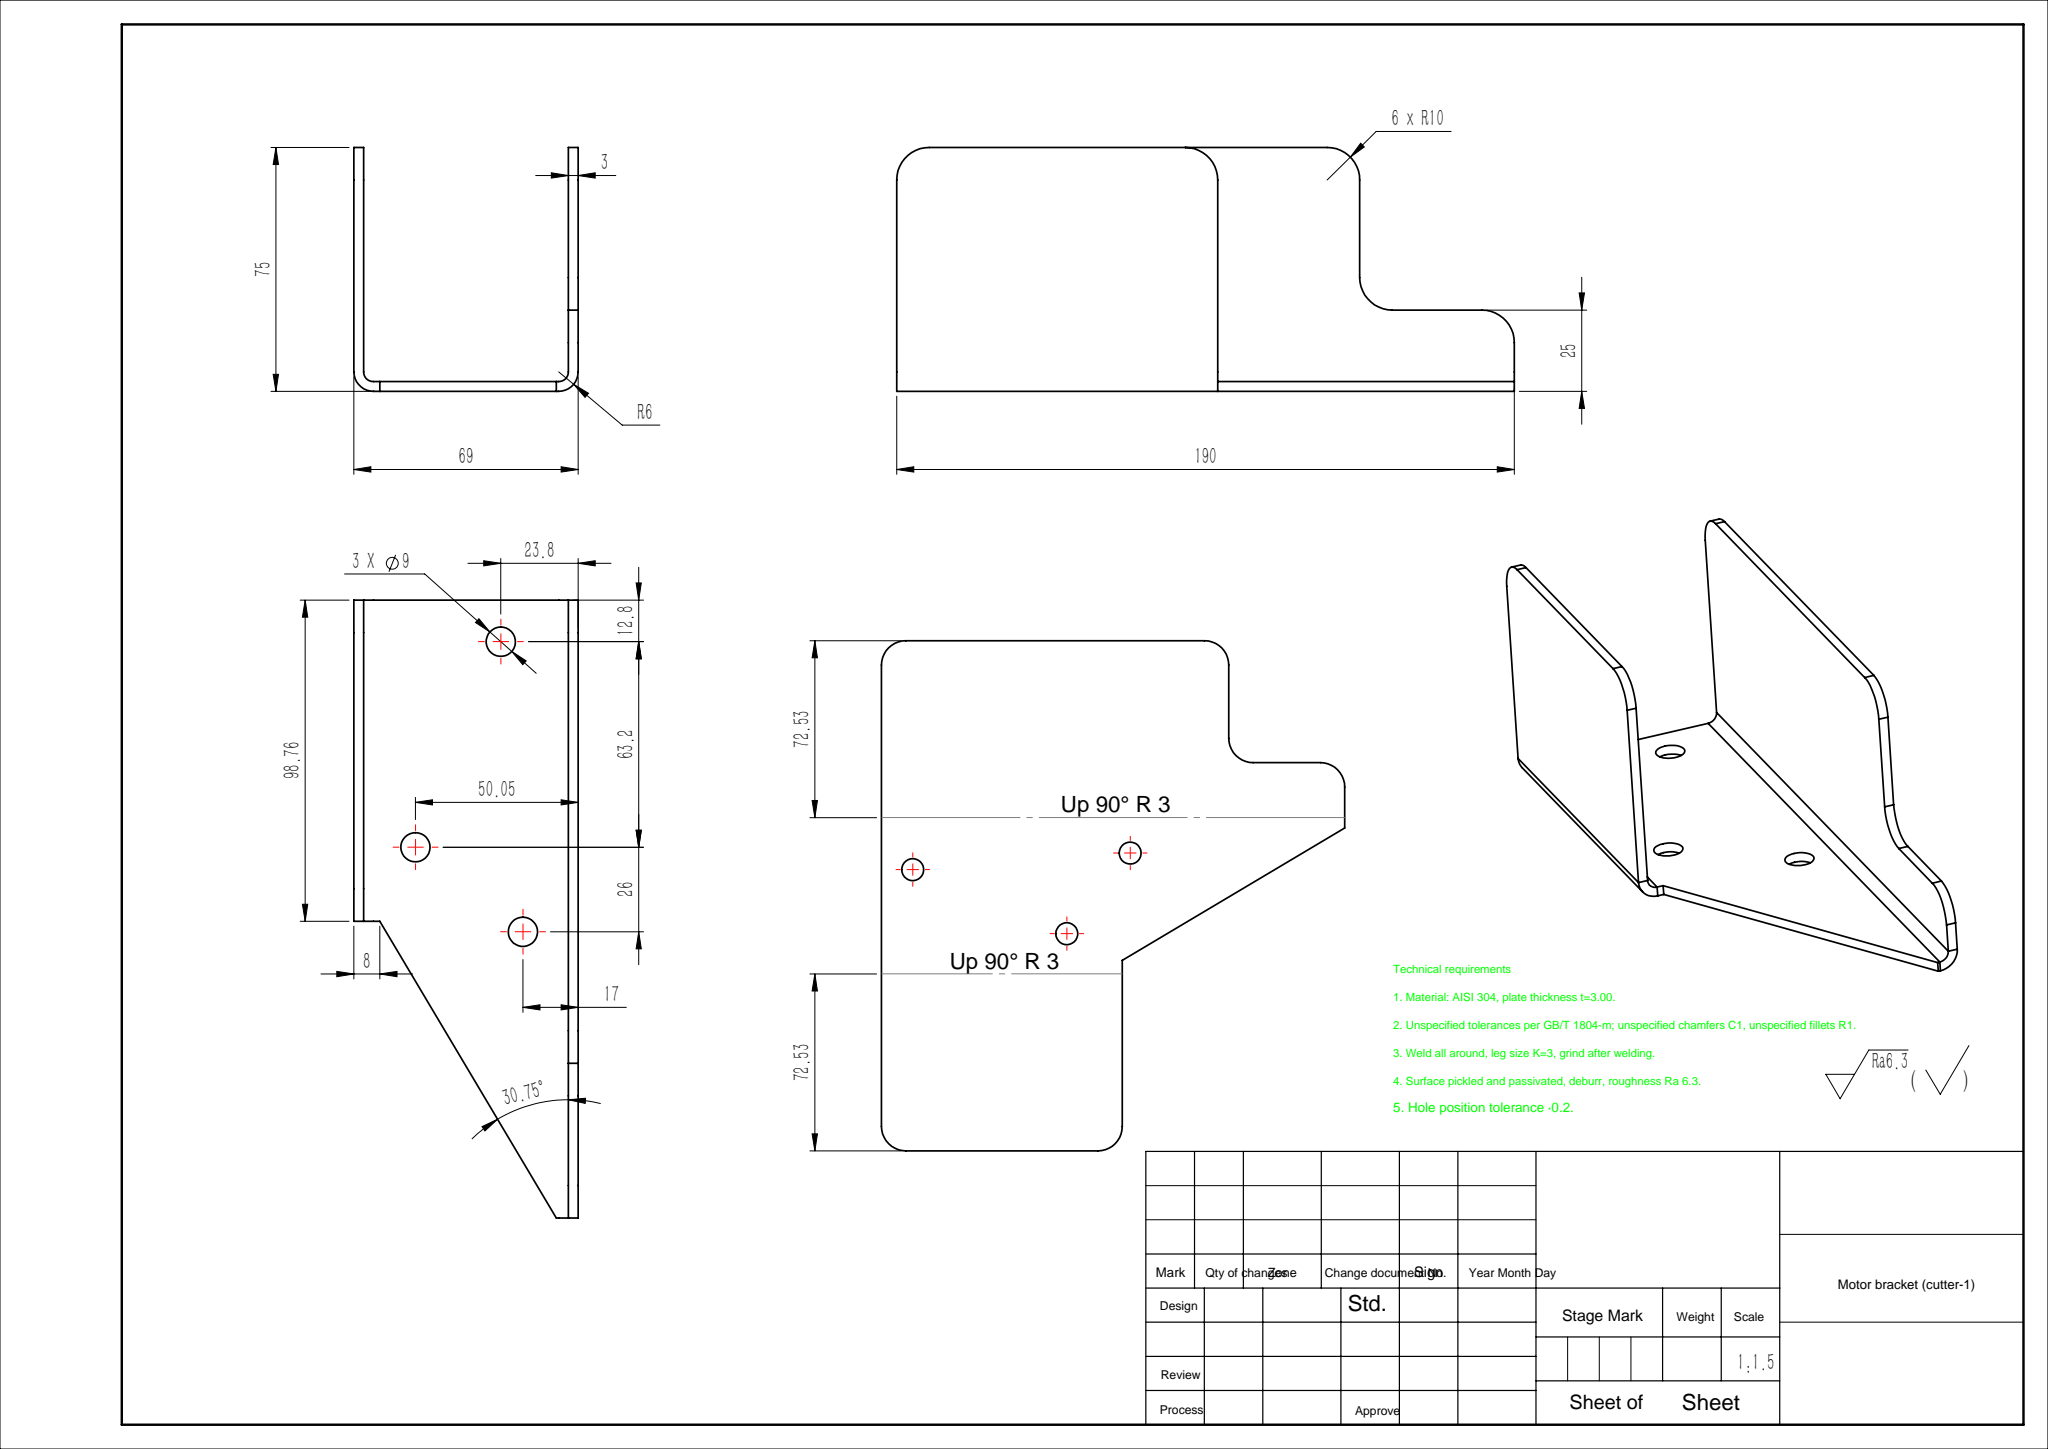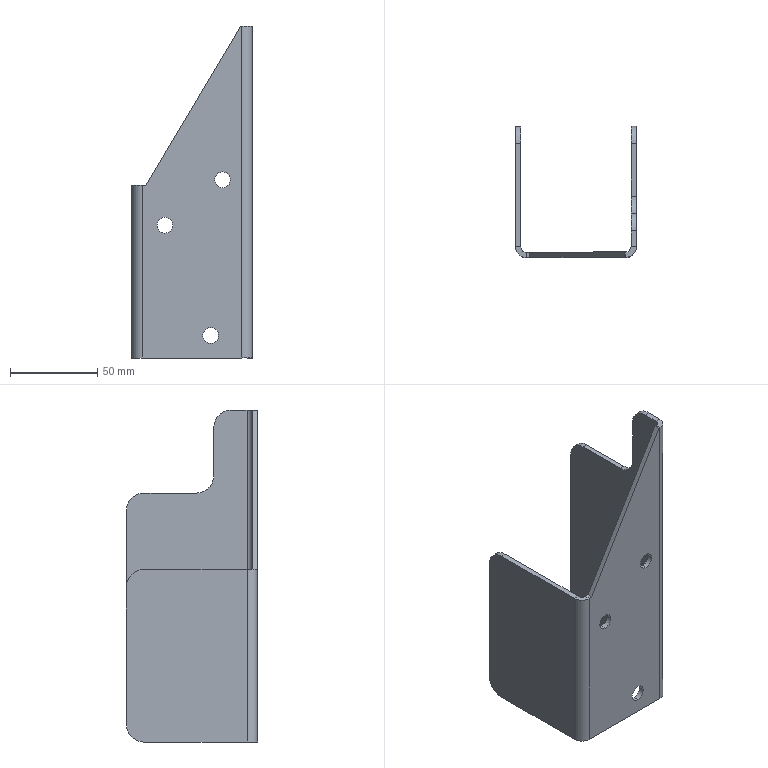Part | SolidWorks | features ICE 3, SMBaseFlange 3, SM3dBend 2, Cut 1, Fillet 1, FlatPattern 1, SheetMetal 1 | 1 solid | 38 faces | box 69 x 75 x 190 mm | volume 82445 mm3 | plane 22 | cylinder 16 | commonest cylinder face diameters 9 x6 20 x6 6 x2 12 x2